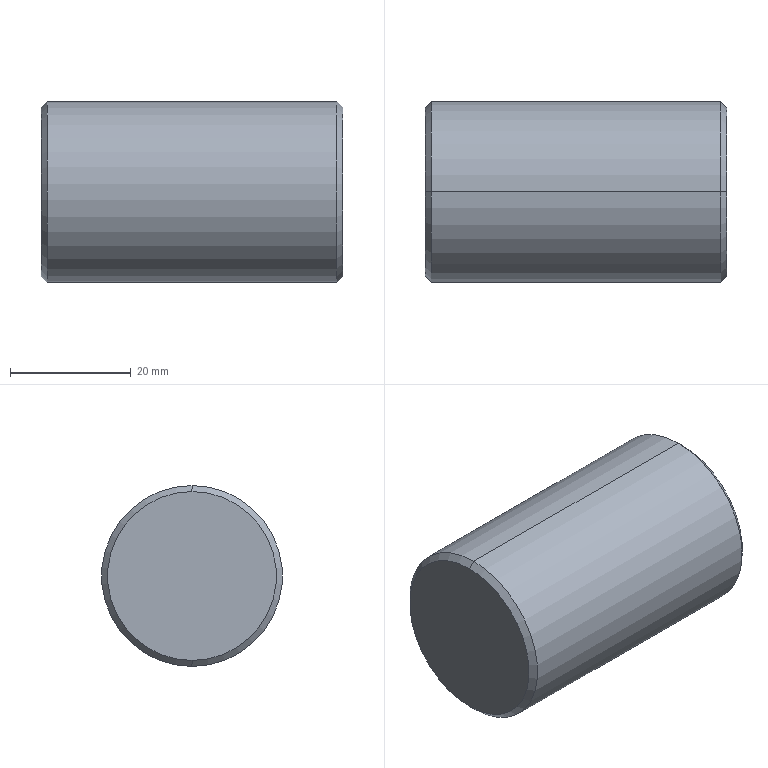Part | SolidWorks | features Chamfer 1, Extrusion 1 | 1 solid | 8 faces | box 50 x 30 x 30 mm | volume 35251 mm3 | cone 4 | cylinder 2 | plane 2 | commonest cylinder face diameters 30 x2
STEP:
#1=CARTESIAN_POINT('',(50.,0.,-14.));
#2=VERTEX_POINT('',#1);
#3=CARTESIAN_POINT('',(50.,0.,14.));
#4=VERTEX_POINT('',#3);
#5=CARTESIAN_POINT('',(50.,0.,0.));
#6=DIRECTION('',(1.,0.,0.));
#7=DIRECTION('',(0.,0.,-1.));
#8=AXIS2_PLACEMENT_3D('',#5,#6,#7);
#9=CIRCLE('',#8,14.);
#10=EDGE_CURVE('',#2,#4,#9,.T.);
#11=ORIENTED_EDGE('',*,*,#10,.F.);
#12=CARTESIAN_POINT('',(49.,0.,-15.));
#13=VERTEX_POINT('',#12);
#14=CARTESIAN_POINT('',(50.,0.,-14.));
#15=DIRECTION('',(-0.7071,0.,-0.7071));
#16=VECTOR('',#15,1000.);
#17=LINE('',#14,#16);
#18=EDGE_CURVE('',#2,#13,#17,.T.);
#19=ORIENTED_EDGE('',*,*,#18,.T.);
#20=CARTESIAN_POINT('',(49.,0.,15.));
#21=VERTEX_POINT('',#20);
#22=CARTESIAN_POINT('',(49.,0.,0.));
#23=DIRECTION('',(-1.,0.,0.));
#24=DIRECTION('',(0.,0.,-1.));
#25=AXIS2_PLACEMENT_3D('',#22,#23,#24);
#26=CIRCLE('',#25,15.);
#27=EDGE_CURVE('',#21,#13,#26,.T.);
#28=ORIENTED_EDGE('',*,*,#27,.F.);
#29=CARTESIAN_POINT('',(50.,0.,14.));
#30=DIRECTION('',(-0.7071,0.,0.7071));
#31=VECTOR('',#30,1000.);
#32=LINE('',#29,#31);
#33=EDGE_CURVE('',#4,#21,#32,.T.);
#34=ORIENTED_EDGE('',*,*,#33,.F.);
#35=EDGE_LOOP('',(#11,#19,#28,#34));
#36=FACE_OUTER_BOUND('',#35,.T.);
#37=CARTESIAN_POINT('',(50.,0.,0.));
#38=DIRECTION('',(-1.,0.,0.));
#39=DIRECTION('',(0.,0.,1.));
#40=AXIS2_PLACEMENT_3D('',#37,#38,#39);
#41=CONICAL_SURFACE('',#40,14.,0.7854);
#42=ADVANCED_FACE('',(#36),#41,.T.);
#43=CARTESIAN_POINT('',(0.,0.,14.));
#44=VERTEX_POINT('',#43);
#45=CARTESIAN_POINT('',(0.,0.,-14.));
#46=VERTEX_POINT('',#45);
#47=CARTESIAN_POINT('',(0.,0.,0.));
#48=DIRECTION('',(-1.,0.,0.));
#49=DIRECTION('',(0.,0.,-1.));
#50=AXIS2_PLACEMENT_3D('',#47,#48,#49);
#51=CIRCLE('',#50,14.);
#52=EDGE_CURVE('',#44,#46,#51,.T.);
#53=ORIENTED_EDGE('',*,*,#52,.F.);
#54=CARTESIAN_POINT('',(1.,0.,15.));
#55=VERTEX_POINT('',#54);
#56=CARTESIAN_POINT('',(1.,0.,15.));
#57=DIRECTION('',(0.7071,0.,0.7071));
#58=VECTOR('',#57,1000.);
#59=LINE('',#56,#58);
#60=EDGE_CURVE('',#44,#55,#59,.T.);
#61=ORIENTED_EDGE('',*,*,#60,.T.);
#62=CARTESIAN_POINT('',(1.,0.,-15.));
#63=VERTEX_POINT('',#62);
#64=CARTESIAN_POINT('',(1.,0.,0.));
#65=DIRECTION('',(1.,0.,0.));
#66=DIRECTION('',(0.,0.,-1.));
#67=AXIS2_PLACEMENT_3D('',#64,#65,#66);
#68=CIRCLE('',#67,15.);
#69=EDGE_CURVE('',#63,#55,#68,.T.);
#70=ORIENTED_EDGE('',*,*,#69,.F.);
#71=CARTESIAN_POINT('',(1.,0.,-15.));
#72=DIRECTION('',(0.7071,0.,-0.7071));
#73=VECTOR('',#72,1000.);
#74=LINE('',#71,#73);
#75=EDGE_CURVE('',#46,#63,#74,.T.);
#76=ORIENTED_EDGE('',*,*,#75,.F.);
#77=EDGE_LOOP('',(#53,#61,#70,#76));
#78=FACE_OUTER_BOUND('',#77,.T.);
#79=CARTESIAN_POINT('',(1.,0.,0.));
#80=DIRECTION('',(1.,0.,0.));
#81=DIRECTION('',(0.,0.,-1.));
#82=AXIS2_PLACEMENT_3D('',#79,#80,#81);
#83=CONICAL_SURFACE('',#82,15.,0.7854);
#84=ADVANCED_FACE('',(#78),#83,.T.);
#85=ORIENTED_EDGE('',*,*,#27,.T.);
#86=CARTESIAN_POINT('',(50.,0.,-15.));
#87=DIRECTION('',(-1.,0.,0.));
#88=VECTOR('',#87,1000.);
#89=LINE('',#86,#88);
#90=EDGE_CURVE('',#13,#63,#89,.T.);
#91=ORIENTED_EDGE('',*,*,#90,.T.);
#92=ORIENTED_EDGE('',*,*,#69,.T.);
#93=CARTESIAN_POINT('',(50.,0.,15.));
#94=DIRECTION('',(-1.,0.,0.));
#95=VECTOR('',#94,1000.);
#96=LINE('',#93,#95);
#97=EDGE_CURVE('',#21,#55,#96,.T.);
#98=ORIENTED_EDGE('',*,*,#97,.F.);
#99=EDGE_LOOP('',(#85,#91,#92,#98));
#100=FACE_OUTER_BOUND('',#99,.T.);
#101=CARTESIAN_POINT('',(50.,0.,0.));
#102=DIRECTION('',(-1.,0.,0.));
#103=DIRECTION('',(0.,0.,1.));
#104=AXIS2_PLACEMENT_3D('',#101,#102,#103);
#105=CYLINDRICAL_SURFACE('',#104,15.);
#106=ADVANCED_FACE('',(#100),#105,.T.);
#107=ORIENTED_EDGE('',*,*,#90,.F.);
#108=CARTESIAN_POINT('',(49.,0.,0.));
#109=DIRECTION('',(-1.,0.,0.));
#110=DIRECTION('',(0.,0.,-1.));
#111=AXIS2_PLACEMENT_3D('',#108,#109,#110);
#112=CIRCLE('',#111,15.);
#113=EDGE_CURVE('',#13,#21,#112,.T.);
#114=ORIENTED_EDGE('',*,*,#113,.T.);
#115=ORIENTED_EDGE('',*,*,#97,.T.);
#116=CARTESIAN_POINT('',(1.,0.,0.));
#117=DIRECTION('',(1.,0.,0.));
#118=DIRECTION('',(0.,0.,-1.));
#119=AXIS2_PLACEMENT_3D('',#116,#117,#118);
#120=CIRCLE('',#119,15.);
#121=EDGE_CURVE('',#55,#63,#120,.T.);
#122=ORIENTED_EDGE('',*,*,#121,.T.);
#123=EDGE_LOOP('',(#107,#114,#115,#122));
#124=FACE_OUTER_BOUND('',#123,.T.);
#125=CARTESIAN_POINT('',(50.,0.,0.));
#126=DIRECTION('',(-1.,0.,0.));
#127=DIRECTION('',(0.,0.,1.));
#128=AXIS2_PLACEMENT_3D('',#125,#126,#127);
#129=CYLINDRICAL_SURFACE('',#128,15.);
#130=ADVANCED_FACE('',(#124),#129,.T.);
#131=CARTESIAN_POINT('',(50.,0.,0.));
#132=DIRECTION('',(1.,0.,0.));
#133=DIRECTION('',(0.,0.,-1.));
#134=AXIS2_PLACEMENT_3D('',#131,#132,#133);
#135=CIRCLE('',#134,14.);
#136=EDGE_CURVE('',#4,#2,#135,.T.);
#137=ORIENTED_EDGE('',*,*,#136,.T.);
#138=ORIENTED_EDGE('',*,*,#10,.T.);
#139=EDGE_LOOP('',(#137,#138));
#140=FACE_OUTER_BOUND('',#139,.T.);
#141=CARTESIAN_POINT('',(50.,0.,0.));
#142=DIRECTION('',(1.,0.,0.));
#143=DIRECTION('',(0.,0.,-1.));
#144=AXIS2_PLACEMENT_3D('',#141,#142,#143);
#145=PLANE('',#144);
#146=ADVANCED_FACE('',(#140),#145,.T.);
#147=CARTESIAN_POINT('',(0.,0.,0.));
#148=DIRECTION('',(-1.,0.,0.));
#149=DIRECTION('',(0.,0.,-1.));
#150=AXIS2_PLACEMENT_3D('',#147,#148,#149);
#151=CIRCLE('',#150,14.);
#152=EDGE_CURVE('',#46,#44,#151,.T.);
#153=ORIENTED_EDGE('',*,*,#152,.T.);
#154=ORIENTED_EDGE('',*,*,#52,.T.);
#155=EDGE_LOOP('',(#153,#154));
#156=FACE_OUTER_BOUND('',#155,.T.);
#157=CARTESIAN_POINT('',(0.,0.,0.));
#158=DIRECTION('',(1.,0.,0.));
#159=DIRECTION('',(0.,0.,-1.));
#160=AXIS2_PLACEMENT_3D('',#157,#158,#159);
#161=PLANE('',#160);
#162=ADVANCED_FACE('',(#156),#161,.F.);
#163=ORIENTED_EDGE('',*,*,#60,.F.);
#164=ORIENTED_EDGE('',*,*,#152,.F.);
#165=ORIENTED_EDGE('',*,*,#75,.T.);
#166=ORIENTED_EDGE('',*,*,#121,.F.);
#167=EDGE_LOOP('',(#163,#164,#165,#166));
#168=FACE_OUTER_BOUND('',#167,.T.);
#169=CARTESIAN_POINT('',(1.,0.,0.));
#170=DIRECTION('',(1.,0.,0.));
#171=DIRECTION('',(0.,0.,-1.));
#172=AXIS2_PLACEMENT_3D('',#169,#170,#171);
#173=CONICAL_SURFACE('',#172,15.,0.7854);
#174=ADVANCED_FACE('',(#168),#173,.T.);
#175=ORIENTED_EDGE('',*,*,#18,.F.);
#176=ORIENTED_EDGE('',*,*,#136,.F.);
#177=ORIENTED_EDGE('',*,*,#33,.T.);
#178=ORIENTED_EDGE('',*,*,#113,.F.);
#179=EDGE_LOOP('',(#175,#176,#177,#178));
#180=FACE_OUTER_BOUND('',#179,.T.);
#181=CARTESIAN_POINT('',(50.,0.,0.));
#182=DIRECTION('',(-1.,0.,0.));
#183=DIRECTION('',(0.,0.,1.));
#184=AXIS2_PLACEMENT_3D('',#181,#182,#183);
#185=CONICAL_SURFACE('',#184,14.,0.7854);
#186=ADVANCED_FACE('',(#180),#185,.T.);
#187=CLOSED_SHELL('',(#42,#84,#106,#130,#146,#162,#174,#186));
#188=MANIFOLD_SOLID_BREP('',#187);
#189=CARTESIAN_POINT('',(0.,0.,0.));
#190=DIRECTION('',(0.,0.,1.));
#191=DIRECTION('',(1.,0.,0.));
#192=AXIS2_PLACEMENT_3D('',#189,#190,#191);
#193=(LENGTH_UNIT()NAMED_UNIT(*)SI_UNIT(.MILLI.,.METRE.));
#194=UNCERTAINTY_MEASURE_WITH_UNIT(LENGTH_MEASURE(0.00001),#193,'','');
#195=(NAMED_UNIT(*)PLANE_ANGLE_UNIT()SI_UNIT($,.RADIAN.));
#196=(NAMED_UNIT(*)SI_UNIT($,.STERADIAN.)SOLID_ANGLE_UNIT());
#197=(GEOMETRIC_REPRESENTATION_CONTEXT(3)GLOBAL_UNCERTAINTY_ASSIGNED_CONTEXT((#194))GLOBAL_UNIT_ASSIGNED_CONTEXT((#193,#195,#196))REPRESENTATION_CONTEXT('',''));
#198=ADVANCED_BREP_SHAPE_REPRESENTATION('',(#188,#192),#197);